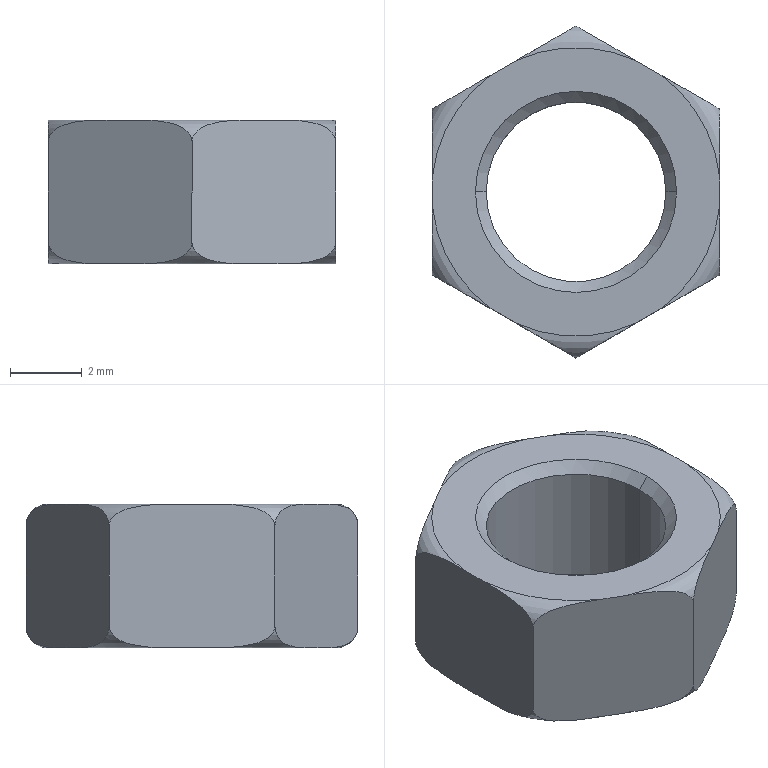Part | NX | features BREP 1 | 1 solid | 26 faces | box 8 x 9.238 x 4 mm | volume 141.214 mm3 | torus 12 | plane 8 | cone 4 | cylinder 2 | commonest cylinder face diameters 5 x2
STEP:
#1=CARTESIAN_POINT('',(2.5,0.,-1.7));
#2=VERTEX_POINT('',#1);
#3=CARTESIAN_POINT('',(-2.5,0.,-1.7));
#4=VERTEX_POINT('',#3);
#5=CARTESIAN_POINT('',(0.,0.,-1.7));
#6=DIRECTION('',(0.,0.,-1.));
#7=DIRECTION('',(-1.,0.,0.));
#8=AXIS2_PLACEMENT_3D('',#5,#6,#7);
#9=CIRCLE('',#8,2.5);
#10=EDGE_CURVE('',#2,#4,#9,.T.);
#11=ORIENTED_EDGE('',*,*,#10,.F.);
#12=CARTESIAN_POINT('',(2.8,0.,-2.));
#13=VERTEX_POINT('',#12);
#14=CARTESIAN_POINT('',(2.8,0.,-2.));
#15=DIRECTION('',(0.7071,0.,-0.7071));
#16=VECTOR('',#15,1000.);
#17=LINE('',#14,#16);
#18=EDGE_CURVE('',#2,#13,#17,.T.);
#19=ORIENTED_EDGE('',*,*,#18,.T.);
#20=CARTESIAN_POINT('',(-2.8,0.,-2.));
#21=VERTEX_POINT('',#20);
#22=CARTESIAN_POINT('',(0.,0.,-2.));
#23=DIRECTION('',(0.,0.,-1.));
#24=DIRECTION('',(-1.,0.,0.));
#25=AXIS2_PLACEMENT_3D('',#22,#23,#24);
#26=CIRCLE('',#25,2.8);
#27=EDGE_CURVE('',#13,#21,#26,.T.);
#28=ORIENTED_EDGE('',*,*,#27,.T.);
#29=CARTESIAN_POINT('',(-2.8,0.,-2.));
#30=DIRECTION('',(-0.7071,0.,-0.7071));
#31=VECTOR('',#30,1000.);
#32=LINE('',#29,#31);
#33=EDGE_CURVE('',#4,#21,#32,.T.);
#34=ORIENTED_EDGE('',*,*,#33,.F.);
#35=EDGE_LOOP('',(#11,#19,#28,#34));
#36=FACE_BOUND('',#35,.T.);
#37=CARTESIAN_POINT('',(0.,0.,-2.));
#38=DIRECTION('',(0.,0.,-1.));
#39=DIRECTION('',(-1.,0.,0.));
#40=AXIS2_PLACEMENT_3D('',#37,#38,#39);
#41=CONICAL_SURFACE('',#40,2.8,0.7854);
#42=ADVANCED_FACE('',(#36),#41,.F.);
#43=CARTESIAN_POINT('',(2.5,0.,1.7));
#44=VERTEX_POINT('',#43);
#45=CARTESIAN_POINT('',(-2.5,0.,1.7));
#46=VERTEX_POINT('',#45);
#47=CARTESIAN_POINT('',(0.,0.,1.7));
#48=DIRECTION('',(0.,0.,-1.));
#49=DIRECTION('',(-1.,0.,0.));
#50=AXIS2_PLACEMENT_3D('',#47,#48,#49);
#51=CIRCLE('',#50,2.5);
#52=EDGE_CURVE('',#44,#46,#51,.T.);
#53=ORIENTED_EDGE('',*,*,#52,.T.);
#54=CARTESIAN_POINT('',(-2.8,0.,2.));
#55=VERTEX_POINT('',#54);
#56=CARTESIAN_POINT('',(-2.5,0.,1.7));
#57=DIRECTION('',(-0.7071,0.,0.7071));
#58=VECTOR('',#57,1000.);
#59=LINE('',#56,#58);
#60=EDGE_CURVE('',#55,#46,#59,.F.);
#61=ORIENTED_EDGE('',*,*,#60,.F.);
#62=CARTESIAN_POINT('',(2.8,0.,2.));
#63=VERTEX_POINT('',#62);
#64=CARTESIAN_POINT('',(0.,0.,2.));
#65=DIRECTION('',(0.,0.,-1.));
#66=DIRECTION('',(-1.,0.,0.));
#67=AXIS2_PLACEMENT_3D('',#64,#65,#66);
#68=CIRCLE('',#67,2.8);
#69=EDGE_CURVE('',#63,#55,#68,.T.);
#70=ORIENTED_EDGE('',*,*,#69,.F.);
#71=CARTESIAN_POINT('',(2.5,0.,1.7));
#72=DIRECTION('',(0.7071,0.,0.7071));
#73=VECTOR('',#72,1000.);
#74=LINE('',#71,#73);
#75=EDGE_CURVE('',#63,#44,#74,.F.);
#76=ORIENTED_EDGE('',*,*,#75,.T.);
#77=EDGE_LOOP('',(#53,#61,#70,#76));
#78=FACE_BOUND('',#77,.T.);
#79=CARTESIAN_POINT('',(0.,0.,1.7));
#80=DIRECTION('',(0.,0.,1.));
#81=DIRECTION('',(1.,0.,0.));
#82=AXIS2_PLACEMENT_3D('',#79,#80,#81);
#83=CONICAL_SURFACE('',#82,2.5,0.7854);
#84=ADVANCED_FACE('',(#78),#83,.F.);
#85=ORIENTED_EDGE('',*,*,#52,.F.);
#86=CARTESIAN_POINT('',(2.5,0.,2.));
#87=DIRECTION('',(0.,0.,-1.));
#88=VECTOR('',#87,1000.);
#89=LINE('',#86,#88);
#90=EDGE_CURVE('',#44,#2,#89,.T.);
#91=ORIENTED_EDGE('',*,*,#90,.T.);
#92=ORIENTED_EDGE('',*,*,#10,.T.);
#93=CARTESIAN_POINT('',(-2.5,0.,2.));
#94=DIRECTION('',(0.,0.,-1.));
#95=VECTOR('',#94,1000.);
#96=LINE('',#93,#95);
#97=EDGE_CURVE('',#46,#4,#96,.T.);
#98=ORIENTED_EDGE('',*,*,#97,.F.);
#99=EDGE_LOOP('',(#85,#91,#92,#98));
#100=FACE_BOUND('',#99,.T.);
#101=CARTESIAN_POINT('',(0.,0.,2.));
#102=DIRECTION('',(0.,0.,-1.));
#103=DIRECTION('',(-1.,0.,0.));
#104=AXIS2_PLACEMENT_3D('',#101,#102,#103);
#105=CYLINDRICAL_SURFACE('',#104,2.5);
#106=ADVANCED_FACE('',(#100),#105,.F.);
#107=CARTESIAN_POINT('',(-2.336,-3.27,-2.));
#108=VERTEX_POINT('',#107);
#109=CARTESIAN_POINT('',(-4.,-0.3883,-2.));
#110=VERTEX_POINT('',#109);
#111=CARTESIAN_POINT('',(0.,0.,-2.));
#112=DIRECTION('',(0.,0.,-1.));
#113=DIRECTION('',(-1.,0.,0.));
#114=AXIS2_PLACEMENT_3D('',#111,#112,#113);
#115=CIRCLE('',#114,4.019);
#116=EDGE_CURVE('',#108,#110,#115,.T.);
#117=ORIENTED_EDGE('',*,*,#116,.T.);
#118=CARTESIAN_POINT('',(-4.,0.3883,-2.));
#119=VERTEX_POINT('',#118);
#120=CARTESIAN_POINT('',(-4.,2.309,-2.));
#121=DIRECTION('',(0.,-1.,0.));
#122=VECTOR('',#121,1000.);
#123=LINE('',#120,#122);
#124=EDGE_CURVE('',#119,#110,#123,.T.);
#125=ORIENTED_EDGE('',*,*,#124,.F.);
#126=CARTESIAN_POINT('',(-2.336,3.27,-2.));
#127=VERTEX_POINT('',#126);
#128=CARTESIAN_POINT('',(0.,0.,-2.));
#129=DIRECTION('',(0.,0.,-1.));
#130=DIRECTION('',(-1.,0.,0.));
#131=AXIS2_PLACEMENT_3D('',#128,#129,#130);
#132=CIRCLE('',#131,4.019);
#133=EDGE_CURVE('',#119,#127,#132,.T.);
#134=ORIENTED_EDGE('',*,*,#133,.T.);
#135=CARTESIAN_POINT('',(-1.664,3.658,-2.));
#136=VERTEX_POINT('',#135);
#137=CARTESIAN_POINT('',(0.,4.619,-2.));
#138=DIRECTION('',(-0.866,-0.5,0.));
#139=VECTOR('',#138,1000.);
#140=LINE('',#137,#139);
#141=EDGE_CURVE('',#136,#127,#140,.T.);
#142=ORIENTED_EDGE('',*,*,#141,.F.);
#143=CARTESIAN_POINT('',(1.664,3.658,-2.));
#144=VERTEX_POINT('',#143);
#145=CARTESIAN_POINT('',(0.,0.,-2.));
#146=DIRECTION('',(0.,0.,-1.));
#147=DIRECTION('',(-1.,0.,0.));
#148=AXIS2_PLACEMENT_3D('',#145,#146,#147);
#149=CIRCLE('',#148,4.019);
#150=EDGE_CURVE('',#136,#144,#149,.T.);
#151=ORIENTED_EDGE('',*,*,#150,.T.);
#152=CARTESIAN_POINT('',(2.336,3.27,-2.));
#153=VERTEX_POINT('',#152);
#154=CARTESIAN_POINT('',(4.,2.309,-2.));
#155=DIRECTION('',(-0.866,0.5,0.));
#156=VECTOR('',#155,1000.);
#157=LINE('',#154,#156);
#158=EDGE_CURVE('',#153,#144,#157,.T.);
#159=ORIENTED_EDGE('',*,*,#158,.F.);
#160=CARTESIAN_POINT('',(4.,0.3883,-2.));
#161=VERTEX_POINT('',#160);
#162=CARTESIAN_POINT('',(0.,0.,-2.));
#163=DIRECTION('',(0.,0.,-1.));
#164=DIRECTION('',(-1.,0.,0.));
#165=AXIS2_PLACEMENT_3D('',#162,#163,#164);
#166=CIRCLE('',#165,4.019);
#167=EDGE_CURVE('',#153,#161,#166,.T.);
#168=ORIENTED_EDGE('',*,*,#167,.T.);
#169=CARTESIAN_POINT('',(4.,-0.3883,-2.));
#170=VERTEX_POINT('',#169);
#171=CARTESIAN_POINT('',(4.,-2.309,-2.));
#172=DIRECTION('',(0.,1.,0.));
#173=VECTOR('',#172,1000.);
#174=LINE('',#171,#173);
#175=EDGE_CURVE('',#170,#161,#174,.T.);
#176=ORIENTED_EDGE('',*,*,#175,.F.);
#177=CARTESIAN_POINT('',(2.336,-3.27,-2.));
#178=VERTEX_POINT('',#177);
#179=CARTESIAN_POINT('',(0.,0.,-2.));
#180=DIRECTION('',(0.,0.,-1.));
#181=DIRECTION('',(-1.,0.,0.));
#182=AXIS2_PLACEMENT_3D('',#179,#180,#181);
#183=CIRCLE('',#182,4.019);
#184=EDGE_CURVE('',#170,#178,#183,.T.);
#185=ORIENTED_EDGE('',*,*,#184,.T.);
#186=CARTESIAN_POINT('',(1.664,-3.658,-2.));
#187=VERTEX_POINT('',#186);
#188=CARTESIAN_POINT('',(0.,-4.619,-2.));
#189=DIRECTION('',(0.866,0.5,0.));
#190=VECTOR('',#189,1000.);
#191=LINE('',#188,#190);
#192=EDGE_CURVE('',#187,#178,#191,.T.);
#193=ORIENTED_EDGE('',*,*,#192,.F.);
#194=CARTESIAN_POINT('',(-1.664,-3.658,-2.));
#195=VERTEX_POINT('',#194);
#196=CARTESIAN_POINT('',(0.,0.,-2.));
#197=DIRECTION('',(0.,0.,-1.));
#198=DIRECTION('',(-1.,0.,0.));
#199=AXIS2_PLACEMENT_3D('',#196,#197,#198);
#200=CIRCLE('',#199,4.019);
#201=EDGE_CURVE('',#187,#195,#200,.T.);
#202=ORIENTED_EDGE('',*,*,#201,.T.);
#203=CARTESIAN_POINT('',(-4.,-2.309,-2.));
#204=DIRECTION('',(0.866,-0.5,0.));
#205=VECTOR('',#204,1000.);
#206=LINE('',#203,#205);
#207=EDGE_CURVE('',#108,#195,#206,.T.);
#208=ORIENTED_EDGE('',*,*,#207,.F.);
#209=EDGE_LOOP('',(#117,#125,#134,#142,#151,#159,#168,#176,#185,#193,#202,#208));
#210=FACE_BOUND('',#209,.T.);
#211=CARTESIAN_POINT('',(0.,0.,-2.));
#212=DIRECTION('',(0.,0.,-1.));
#213=DIRECTION('',(-1.,0.,0.));
#214=AXIS2_PLACEMENT_3D('',#211,#212,#213);
#215=CIRCLE('',#214,2.8);
#216=EDGE_CURVE('',#21,#13,#215,.T.);
#217=ORIENTED_EDGE('',*,*,#216,.F.);
#218=ORIENTED_EDGE('',*,*,#27,.F.);
#219=EDGE_LOOP('',(#217,#218));
#220=FACE_BOUND('',#219,.T.);
#221=CARTESIAN_POINT('',(-4.,6.928,-2.));
#222=DIRECTION('',(0.,0.,1.));
#223=DIRECTION('',(1.,0.,0.));
#224=AXIS2_PLACEMENT_3D('',#221,#222,#223);
#225=PLANE('',#224);
#226=ADVANCED_FACE('',(#210,#220),#225,.F.);
#227=CARTESIAN_POINT('',(-4.,0.3883,2.));
#228=VERTEX_POINT('',#227);
#229=CARTESIAN_POINT('',(-4.,-0.3883,2.));
#230=VERTEX_POINT('',#229);
#231=CARTESIAN_POINT('',(-4.,2.309,2.));
#232=DIRECTION('',(0.,-1.,0.));
#233=VECTOR('',#232,1000.);
#234=LINE('',#231,#233);
#235=EDGE_CURVE('',#228,#230,#234,.T.);
#236=ORIENTED_EDGE('',*,*,#235,.T.);
#237=CARTESIAN_POINT('',(-2.336,-3.27,2.));
#238=VERTEX_POINT('',#237);
#239=CARTESIAN_POINT('',(0.,0.,2.));
#240=DIRECTION('',(0.,0.,-1.));
#241=DIRECTION('',(-1.,0.,0.));
#242=AXIS2_PLACEMENT_3D('',#239,#240,#241);
#243=CIRCLE('',#242,4.019);
#244=EDGE_CURVE('',#238,#230,#243,.T.);
#245=ORIENTED_EDGE('',*,*,#244,.F.);
#246=CARTESIAN_POINT('',(-1.664,-3.658,2.));
#247=VERTEX_POINT('',#246);
#248=CARTESIAN_POINT('',(-4.,-2.309,2.));
#249=DIRECTION('',(0.866,-0.5,0.));
#250=VECTOR('',#249,1000.);
#251=LINE('',#248,#250);
#252=EDGE_CURVE('',#238,#247,#251,.T.);
#253=ORIENTED_EDGE('',*,*,#252,.T.);
#254=CARTESIAN_POINT('',(1.664,-3.658,2.));
#255=VERTEX_POINT('',#254);
#256=CARTESIAN_POINT('',(0.,0.,2.));
#257=DIRECTION('',(0.,0.,-1.));
#258=DIRECTION('',(-1.,0.,0.));
#259=AXIS2_PLACEMENT_3D('',#256,#257,#258);
#260=CIRCLE('',#259,4.019);
#261=EDGE_CURVE('',#255,#247,#260,.T.);
#262=ORIENTED_EDGE('',*,*,#261,.F.);
#263=CARTESIAN_POINT('',(2.336,-3.27,2.));
#264=VERTEX_POINT('',#263);
#265=CARTESIAN_POINT('',(0.,-4.619,2.));
#266=DIRECTION('',(0.866,0.5,0.));
#267=VECTOR('',#266,1000.);
#268=LINE('',#265,#267);
#269=EDGE_CURVE('',#255,#264,#268,.T.);
#270=ORIENTED_EDGE('',*,*,#269,.T.);
#271=CARTESIAN_POINT('',(4.,-0.3883,2.));
#272=VERTEX_POINT('',#271);
#273=CARTESIAN_POINT('',(0.,0.,2.));
#274=DIRECTION('',(0.,0.,-1.));
#275=DIRECTION('',(-1.,0.,0.));
#276=AXIS2_PLACEMENT_3D('',#273,#274,#275);
#277=CIRCLE('',#276,4.019);
#278=EDGE_CURVE('',#272,#264,#277,.T.);
#279=ORIENTED_EDGE('',*,*,#278,.F.);
#280=CARTESIAN_POINT('',(4.,0.3883,2.));
#281=VERTEX_POINT('',#280);
#282=CARTESIAN_POINT('',(4.,-2.309,2.));
#283=DIRECTION('',(0.,1.,0.));
#284=VECTOR('',#283,1000.);
#285=LINE('',#282,#284);
#286=EDGE_CURVE('',#272,#281,#285,.T.);
#287=ORIENTED_EDGE('',*,*,#286,.T.);
#288=CARTESIAN_POINT('',(2.336,3.27,2.));
#289=VERTEX_POINT('',#288);
#290=CARTESIAN_POINT('',(0.,0.,2.));
#291=DIRECTION('',(0.,0.,-1.));
#292=DIRECTION('',(-1.,0.,0.));
#293=AXIS2_PLACEMENT_3D('',#290,#291,#292);
#294=CIRCLE('',#293,4.019);
#295=EDGE_CURVE('',#289,#281,#294,.T.);
#296=ORIENTED_EDGE('',*,*,#295,.F.);
#297=CARTESIAN_POINT('',(1.664,3.658,2.));
#298=VERTEX_POINT('',#297);
#299=CARTESIAN_POINT('',(4.,2.309,2.));
#300=DIRECTION('',(-0.866,0.5,0.));
#301=VECTOR('',#300,1000.);
#302=LINE('',#299,#301);
#303=EDGE_CURVE('',#289,#298,#302,.T.);
#304=ORIENTED_EDGE('',*,*,#303,.T.);
#305=CARTESIAN_POINT('',(-1.664,3.658,2.));
#306=VERTEX_POINT('',#305);
#307=CARTESIAN_POINT('',(0.,0.,2.));
#308=DIRECTION('',(0.,0.,-1.));
#309=DIRECTION('',(-1.,0.,0.));
#310=AXIS2_PLACEMENT_3D('',#307,#308,#309);
#311=CIRCLE('',#310,4.019);
#312=EDGE_CURVE('',#306,#298,#311,.T.);
#313=ORIENTED_EDGE('',*,*,#312,.F.);
#314=CARTESIAN_POINT('',(-2.336,3.27,2.));
#315=VERTEX_POINT('',#314);
#316=CARTESIAN_POINT('',(0.,4.619,2.));
#317=DIRECTION('',(-0.866,-0.5,0.));
#318=VECTOR('',#317,1000.);
#319=LINE('',#316,#318);
#320=EDGE_CURVE('',#306,#315,#319,.T.);
#321=ORIENTED_EDGE('',*,*,#320,.T.);
#322=CARTESIAN_POINT('',(0.,0.,2.));
#323=DIRECTION('',(0.,0.,-1.));
#324=DIRECTION('',(-1.,0.,0.));
#325=AXIS2_PLACEMENT_3D('',#322,#323,#324);
#326=CIRCLE('',#325,4.019);
#327=EDGE_CURVE('',#228,#315,#326,.T.);
#328=ORIENTED_EDGE('',*,*,#327,.F.);
#329=EDGE_LOOP('',(#236,#245,#253,#262,#270,#279,#287,#296,#304,#313,#321,#328));
#330=FACE_BOUND('',#329,.T.);
#331=ORIENTED_EDGE('',*,*,#69,.T.);
#332=CARTESIAN_POINT('',(0.,0.,2.));
#333=DIRECTION('',(0.,0.,-1.));
#334=DIRECTION('',(-1.,0.,0.));
#335=AXIS2_PLACEMENT_3D('',#332,#333,#334);
#336=CIRCLE('',#335,2.8);
#337=EDGE_CURVE('',#55,#63,#336,.T.);
#338=ORIENTED_EDGE('',*,*,#337,.T.);
#339=EDGE_LOOP('',(#331,#338));
#340=FACE_BOUND('',#339,.T.);
#341=CARTESIAN_POINT('',(-4.,6.928,2.));
#342=DIRECTION('',(0.,0.,1.));
#343=DIRECTION('',(1.,0.,0.));
#344=AXIS2_PLACEMENT_3D('',#341,#342,#343);
#345=PLANE('',#344);
#346=ADVANCED_FACE('',(#330,#340),#345,.T.);
#347=CARTESIAN_POINT('',(4.,2.309,1.4));
#348=VERTEX_POINT('',#347);
#349=CARTESIAN_POINT('',(4.,2.309,-1.4));
#350=VERTEX_POINT('',#349);
#351=CARTESIAN_POINT('',(4.,2.309,2.));
#352=DIRECTION('',(0.,0.,-1.));
#353=VECTOR('',#352,1000.);
#354=LINE('',#351,#353);
#355=EDGE_CURVE('',#348,#350,#354,.T.);
#356=ORIENTED_EDGE('',*,*,#355,.T.);
#357=CARTESIAN_POINT('',(4.,2.309,-1.4));
#358=CARTESIAN_POINT('',(4.,2.309,-1.575));
#359=CARTESIAN_POINT('',(3.769,2.443,-1.795));
#360=CARTESIAN_POINT('',(3.536,2.578,-1.889));
#361=CARTESIAN_POINT('',(3.249,2.743,-1.958));
#362=CARTESIAN_POINT('',(3.077,2.842,-1.977));
#363=CARTESIAN_POINT('',(2.78,3.014,-1.996));
#364=CARTESIAN_POINT('',(2.625,3.103,-1.998));
#365=CARTESIAN_POINT('',(2.437,3.212,-2.));
#366=CARTESIAN_POINT('',(2.336,3.27,-2.));
#367=B_SPLINE_CURVE_WITH_KNOTS('',3,(#357,#358,#359,#360,#361,#362,#363,#364,#365,#366),.UNSPECIFIED.,.F.,.F.,(4,1,1,1,1,1,1,4),(0.,0.25,0.375,0.5,0.625,0.75,0.875,1.),.UNSPECIFIED.);
#368=EDGE_CURVE('',#350,#153,#367,.T.);
#369=ORIENTED_EDGE('',*,*,#368,.T.);
#370=ORIENTED_EDGE('',*,*,#158,.T.);
#371=CARTESIAN_POINT('',(0.,4.619,-1.4));
#372=VERTEX_POINT('',#371);
#373=CARTESIAN_POINT('',(1.664,3.658,-2.));
#374=CARTESIAN_POINT('',(1.463,3.774,-2.));
#375=CARTESIAN_POINT('',(1.304,3.866,-2.002));
#376=CARTESIAN_POINT('',(0.9254,4.085,-1.978));
#377=CARTESIAN_POINT('',(0.7461,4.188,-1.957));
#378=CARTESIAN_POINT('',(0.4638,4.351,-1.889));
#379=CARTESIAN_POINT('',(0.2273,4.488,-1.792));
#380=CARTESIAN_POINT('',(0.,4.619,-1.577));
#381=CARTESIAN_POINT('',(0.,4.619,-1.4));
#382=B_SPLINE_CURVE_WITH_KNOTS('',3,(#373,#374,#375,#376,#377,#378,#379,#380,#381),.UNSPECIFIED.,.F.,.F.,(4,1,1,1,1,1,4),(0.,0.25,0.375,0.5,0.625,0.75,1.),.UNSPECIFIED.);
#383=EDGE_CURVE('',#144,#372,#382,.T.);
#384=ORIENTED_EDGE('',*,*,#383,.T.);
#385=CARTESIAN_POINT('',(0.,4.619,1.4));
#386=VERTEX_POINT('',#385);
#387=CARTESIAN_POINT('',(0.,4.619,2.));
#388=DIRECTION('',(0.,0.,-1.));
#389=VECTOR('',#388,1000.);
#390=LINE('',#387,#389);
#391=EDGE_CURVE('',#386,#372,#390,.T.);
#392=ORIENTED_EDGE('',*,*,#391,.F.);
#393=CARTESIAN_POINT('',(0.,4.619,1.4));
#394=CARTESIAN_POINT('',(0.,4.619,1.575));
#395=CARTESIAN_POINT('',(0.2312,4.485,1.795));
#396=CARTESIAN_POINT('',(0.4644,4.351,1.889));
#397=CARTESIAN_POINT('',(0.7506,4.185,1.958));
#398=CARTESIAN_POINT('',(0.9231,4.086,1.977));
#399=CARTESIAN_POINT('',(1.22,3.915,1.996));
#400=CARTESIAN_POINT('',(1.375,3.825,1.998));
#401=CARTESIAN_POINT('',(1.563,3.716,2.));
#402=CARTESIAN_POINT('',(1.664,3.658,2.));
#403=B_SPLINE_CURVE_WITH_KNOTS('',3,(#393,#394,#395,#396,#397,#398,#399,#400,#401,#402),.UNSPECIFIED.,.F.,.F.,(4,1,1,1,1,1,1,4),(0.,0.25,0.375,0.5,0.625,0.75,0.875,1.),.UNSPECIFIED.);
#404=EDGE_CURVE('',#386,#298,#403,.T.);
#405=ORIENTED_EDGE('',*,*,#404,.T.);
#406=ORIENTED_EDGE('',*,*,#303,.F.);
#407=CARTESIAN_POINT('',(2.336,3.27,2.));
#408=CARTESIAN_POINT('',(2.537,3.154,2.));
#409=CARTESIAN_POINT('',(2.696,3.062,2.002));
#410=CARTESIAN_POINT('',(3.075,2.844,1.978));
#411=CARTESIAN_POINT('',(3.254,2.74,1.957));
#412=CARTESIAN_POINT('',(3.536,2.577,1.889));
#413=CARTESIAN_POINT('',(3.773,2.441,1.792));
#414=CARTESIAN_POINT('',(4.,2.309,1.577));
#415=CARTESIAN_POINT('',(4.,2.309,1.4));
#416=B_SPLINE_CURVE_WITH_KNOTS('',3,(#407,#408,#409,#410,#411,#412,#413,#414,#415),.UNSPECIFIED.,.F.,.F.,(4,1,1,1,1,1,4),(0.,0.25,0.375,0.5,0.625,0.75,1.),.UNSPECIFIED.);
#417=EDGE_CURVE('',#289,#348,#416,.T.);
#418=ORIENTED_EDGE('',*,*,#417,.T.);
#419=EDGE_LOOP('',(#356,#369,#370,#384,#392,#405,#406,#418));
#420=FACE_BOUND('',#419,.T.);
#421=CARTESIAN_POINT('',(4.,2.309,2.));
#422=DIRECTION('',(-0.5,-0.866,0.));
#423=DIRECTION('',(-0.866,0.5,0.));
#424=AXIS2_PLACEMENT_3D('',#421,#422,#423);
#425=PLANE('',#424);
#426=ADVANCED_FACE('',(#420),#425,.F.);
#427=ORIENTED_EDGE('',*,*,#391,.T.);
#428=CARTESIAN_POINT('',(0.,4.619,-1.4));
#429=CARTESIAN_POINT('',(0.,4.619,-1.575));
#430=CARTESIAN_POINT('',(-0.2312,4.485,-1.795));
#431=CARTESIAN_POINT('',(-0.4644,4.351,-1.889));
#432=CARTESIAN_POINT('',(-0.7506,4.185,-1.958));
#433=CARTESIAN_POINT('',(-0.9231,4.086,-1.977));
#434=CARTESIAN_POINT('',(-1.22,3.915,-1.996));
#435=CARTESIAN_POINT('',(-1.375,3.825,-1.998));
#436=CARTESIAN_POINT('',(-1.563,3.716,-2.));
#437=CARTESIAN_POINT('',(-1.664,3.658,-2.));
#438=B_SPLINE_CURVE_WITH_KNOTS('',3,(#428,#429,#430,#431,#432,#433,#434,#435,#436,#437),.UNSPECIFIED.,.F.,.F.,(4,1,1,1,1,1,1,4),(0.,0.25,0.375,0.5,0.625,0.75,0.875,1.),.UNSPECIFIED.);
#439=EDGE_CURVE('',#372,#136,#438,.T.);
#440=ORIENTED_EDGE('',*,*,#439,.T.);
#441=ORIENTED_EDGE('',*,*,#141,.T.);
#442=CARTESIAN_POINT('',(-4.,2.309,-1.4));
#443=VERTEX_POINT('',#442);
#444=CARTESIAN_POINT('',(-2.336,3.27,-2.));
#445=CARTESIAN_POINT('',(-2.537,3.154,-2.));
#446=CARTESIAN_POINT('',(-2.696,3.062,-2.002));
#447=CARTESIAN_POINT('',(-3.075,2.844,-1.978));
#448=CARTESIAN_POINT('',(-3.254,2.74,-1.957));
#449=CARTESIAN_POINT('',(-3.536,2.577,-1.889));
#450=CARTESIAN_POINT('',(-3.773,2.441,-1.792));
#451=CARTESIAN_POINT('',(-4.,2.309,-1.577));
#452=CARTESIAN_POINT('',(-4.,2.309,-1.4));
#453=B_SPLINE_CURVE_WITH_KNOTS('',3,(#444,#445,#446,#447,#448,#449,#450,#451,#452),.UNSPECIFIED.,.F.,.F.,(4,1,1,1,1,1,4),(0.,0.25,0.375,0.5,0.625,0.75,1.),.UNSPECIFIED.);
#454=EDGE_CURVE('',#127,#443,#453,.T.);
#455=ORIENTED_EDGE('',*,*,#454,.T.);
#456=CARTESIAN_POINT('',(-4.,2.309,1.4));
#457=VERTEX_POINT('',#456);
#458=CARTESIAN_POINT('',(-4.,2.309,2.));
#459=DIRECTION('',(0.,0.,-1.));
#460=VECTOR('',#459,1000.);
#461=LINE('',#458,#460);
#462=EDGE_CURVE('',#457,#443,#461,.T.);
#463=ORIENTED_EDGE('',*,*,#462,.F.);
#464=CARTESIAN_POINT('',(-4.,2.309,1.4));
#465=CARTESIAN_POINT('',(-4.,2.309,1.575));
#466=CARTESIAN_POINT('',(-3.769,2.443,1.795));
#467=CARTESIAN_POINT('',(-3.536,2.578,1.889));
#468=CARTESIAN_POINT('',(-3.249,2.743,1.958));
#469=CARTESIAN_POINT('',(-3.077,2.842,1.977));
#470=CARTESIAN_POINT('',(-2.78,3.014,1.996));
#471=CARTESIAN_POINT('',(-2.625,3.103,1.998));
#472=CARTESIAN_POINT('',(-2.437,3.212,2.));
#473=CARTESIAN_POINT('',(-2.336,3.27,2.));
#474=B_SPLINE_CURVE_WITH_KNOTS('',3,(#464,#465,#466,#467,#468,#469,#470,#471,#472,#473),.UNSPECIFIED.,.F.,.F.,(4,1,1,1,1,1,1,4),(0.,0.25,0.375,0.5,0.625,0.75,0.875,1.),.UNSPECIFIED.);
#475=EDGE_CURVE('',#457,#315,#474,.T.);
#476=ORIENTED_EDGE('',*,*,#475,.T.);
#477=ORIENTED_EDGE('',*,*,#320,.F.);
#478=CARTESIAN_POINT('',(-1.664,3.658,2.));
#479=CARTESIAN_POINT('',(-1.463,3.774,2.));
#480=CARTESIAN_POINT('',(-1.304,3.866,2.002));
#481=CARTESIAN_POINT('',(-0.9254,4.085,1.978));
#482=CARTESIAN_POINT('',(-0.7461,4.188,1.957));
#483=CARTESIAN_POINT('',(-0.4638,4.351,1.889));
#484=CARTESIAN_POINT('',(-0.2273,4.488,1.792));
#485=CARTESIAN_POINT('',(0.,4.619,1.577));
#486=CARTESIAN_POINT('',(0.,4.619,1.4));
#487=B_SPLINE_CURVE_WITH_KNOTS('',3,(#478,#479,#480,#481,#482,#483,#484,#485,#486),.UNSPECIFIED.,.F.,.F.,(4,1,1,1,1,1,4),(0.,0.25,0.375,0.5,0.625,0.75,1.),.UNSPECIFIED.);
#488=EDGE_CURVE('',#306,#386,#487,.T.);
#489=ORIENTED_EDGE('',*,*,#488,.T.);
#490=EDGE_LOOP('',(#427,#440,#441,#455,#463,#476,#477,#489));
#491=FACE_BOUND('',#490,.T.);
#492=CARTESIAN_POINT('',(0.,4.619,2.));
#493=DIRECTION('',(0.5,-0.866,0.));
#494=DIRECTION('',(0.,0.,-1.));
#495=AXIS2_PLACEMENT_3D('',#492,#493,#494);
#496=PLANE('',#495);
#497=ADVANCED_FACE('',(#491),#496,.F.);
#498=ORIENTED_EDGE('',*,*,#124,.T.);
#499=CARTESIAN_POINT('',(-4.,-2.309,-1.4));
#500=VERTEX_POINT('',#499);
#501=CARTESIAN_POINT('',(-4.,-0.3883,-2.));
#502=CARTESIAN_POINT('',(-4.,-0.6198,-2.));
#503=CARTESIAN_POINT('',(-4.,-0.8035,-2.002));
#504=CARTESIAN_POINT('',(-4.,-1.24,-1.978));
#505=CARTESIAN_POINT('',(-4.,-1.447,-1.957));
#506=CARTESIAN_POINT('',(-4.,-1.774,-1.889));
#507=CARTESIAN_POINT('',(-4.,-2.047,-1.793));
#508=CARTESIAN_POINT('',(-4.,-2.309,-1.573));
#509=CARTESIAN_POINT('',(-4.,-2.309,-1.4));
#510=B_SPLINE_CURVE_WITH_KNOTS('',3,(#501,#502,#503,#504,#505,#506,#507,#508,#509),.UNSPECIFIED.,.F.,.F.,(4,1,1,1,1,1,4),(0.,0.25,0.375,0.5,0.625,0.75,1.),.UNSPECIFIED.);
#511=EDGE_CURVE('',#110,#500,#510,.T.);
#512=ORIENTED_EDGE('',*,*,#511,.T.);
#513=CARTESIAN_POINT('',(-4.,-2.309,1.4));
#514=VERTEX_POINT('',#513);
#515=CARTESIAN_POINT('',(-4.,-2.309,2.));
#516=DIRECTION('',(0.,0.,-1.));
#517=VECTOR('',#516,1000.);
#518=LINE('',#515,#517);
#519=EDGE_CURVE('',#514,#500,#518,.T.);
#520=ORIENTED_EDGE('',*,*,#519,.F.);
#521=CARTESIAN_POINT('',(-4.,-2.309,1.4));
#522=CARTESIAN_POINT('',(-4.,-2.309,1.573));
#523=CARTESIAN_POINT('',(-4.,-2.041,1.796));
#524=CARTESIAN_POINT('',(-4.,-1.771,1.89));
#525=CARTESIAN_POINT('',(-4.,-1.438,1.958));
#526=CARTESIAN_POINT('',(-4.,-1.241,1.978));
#527=CARTESIAN_POINT('',(-4.,-0.8989,1.997));
#528=CARTESIAN_POINT('',(-4.,-0.7208,1.998));
#529=CARTESIAN_POINT('',(-4.,-0.504,2.));
#530=CARTESIAN_POINT('',(-4.,-0.3883,2.));
#531=B_SPLINE_CURVE_WITH_KNOTS('',3,(#521,#522,#523,#524,#525,#526,#527,#528,#529,#530),.UNSPECIFIED.,.F.,.F.,(4,1,1,1,1,1,1,4),(0.,0.25,0.375,0.5,0.625,0.75,0.875,1.),.UNSPECIFIED.);
#532=EDGE_CURVE('',#514,#230,#531,.T.);
#533=ORIENTED_EDGE('',*,*,#532,.T.);
#534=ORIENTED_EDGE('',*,*,#235,.F.);
#535=CARTESIAN_POINT('',(-4.,0.3883,2.));
#536=CARTESIAN_POINT('',(-4.,0.6198,2.));
#537=CARTESIAN_POINT('',(-4.,0.8035,2.002));
#538=CARTESIAN_POINT('',(-4.,1.24,1.978));
#539=CARTESIAN_POINT('',(-4.,1.447,1.957));
#540=CARTESIAN_POINT('',(-4.,1.774,1.889));
#541=CARTESIAN_POINT('',(-4.,2.047,1.793));
#542=CARTESIAN_POINT('',(-4.,2.309,1.573));
#543=CARTESIAN_POINT('',(-4.,2.309,1.4));
#544=B_SPLINE_CURVE_WITH_KNOTS('',3,(#535,#536,#537,#538,#539,#540,#541,#542,#543),.UNSPECIFIED.,.F.,.F.,(4,1,1,1,1,1,4),(0.,0.25,0.375,0.5,0.625,0.75,1.),.UNSPECIFIED.);
#545=EDGE_CURVE('',#228,#457,#544,.T.);
#546=ORIENTED_EDGE('',*,*,#545,.T.);
#547=ORIENTED_EDGE('',*,*,#462,.T.);
#548=CARTESIAN_POINT('',(-4.,2.309,-1.4));
#549=CARTESIAN_POINT('',(-4.,2.309,-1.573));
#550=CARTESIAN_POINT('',(-4.,2.041,-1.796));
#551=CARTESIAN_POINT('',(-4.,1.771,-1.89));
#552=CARTESIAN_POINT('',(-4.,1.438,-1.958));
#553=CARTESIAN_POINT('',(-4.,1.241,-1.978));
#554=CARTESIAN_POINT('',(-4.,0.8989,-1.997));
#555=CARTESIAN_POINT('',(-4.,0.7208,-1.998));
#556=CARTESIAN_POINT('',(-4.,0.504,-2.));
#557=CARTESIAN_POINT('',(-4.,0.3883,-2.));
#558=B_SPLINE_CURVE_WITH_KNOTS('',3,(#548,#549,#550,#551,#552,#553,#554,#555,#556,#557),.UNSPECIFIED.,.F.,.F.,(4,1,1,1,1,1,1,4),(0.,0.25,0.375,0.5,0.625,0.75,0.875,1.),.UNSPECIFIED.);
#559=EDGE_CURVE('',#443,#119,#558,.T.);
#560=ORIENTED_EDGE('',*,*,#559,.T.);
#561=EDGE_LOOP('',(#498,#512,#520,#533,#534,#546,#547,#560));
#562=FACE_BOUND('',#561,.T.);
#563=CARTESIAN_POINT('',(-4.,2.309,2.));
#564=DIRECTION('',(1.,0.,0.));
#565=DIRECTION('',(0.,1.,0.));
#566=AXIS2_PLACEMENT_3D('',#563,#564,#565);
#567=PLANE('',#566);
#568=ADVANCED_FACE('',(#562),#567,.F.);
#569=ORIENTED_EDGE('',*,*,#519,.T.);
#570=CARTESIAN_POINT('',(-4.,-2.309,-1.4));
#571=CARTESIAN_POINT('',(-4.,-2.309,-1.575));
#572=CARTESIAN_POINT('',(-3.769,-2.443,-1.795));
#573=CARTESIAN_POINT('',(-3.536,-2.578,-1.889));
#574=CARTESIAN_POINT('',(-3.249,-2.743,-1.958));
#575=CARTESIAN_POINT('',(-3.077,-2.842,-1.977));
#576=CARTESIAN_POINT('',(-2.78,-3.014,-1.996));
#577=CARTESIAN_POINT('',(-2.625,-3.103,-1.998));
#578=CARTESIAN_POINT('',(-2.437,-3.212,-2.));
#579=CARTESIAN_POINT('',(-2.336,-3.27,-2.));
#580=B_SPLINE_CURVE_WITH_KNOTS('',3,(#570,#571,#572,#573,#574,#575,#576,#577,#578,#579),.UNSPECIFIED.,.F.,.F.,(4,1,1,1,1,1,1,4),(0.,0.25,0.375,0.5,0.625,0.75,0.875,1.),.UNSPECIFIED.);
#581=EDGE_CURVE('',#500,#108,#580,.T.);
#582=ORIENTED_EDGE('',*,*,#581,.T.);
#583=ORIENTED_EDGE('',*,*,#207,.T.);
#584=CARTESIAN_POINT('',(0.,-4.619,-1.4));
#585=VERTEX_POINT('',#584);
#586=CARTESIAN_POINT('',(-1.664,-3.658,-2.));
#587=CARTESIAN_POINT('',(-1.463,-3.774,-2.));
#588=CARTESIAN_POINT('',(-1.304,-3.866,-2.002));
#589=CARTESIAN_POINT('',(-0.9254,-4.085,-1.978));
#590=CARTESIAN_POINT('',(-0.7461,-4.188,-1.957));
#591=CARTESIAN_POINT('',(-0.4638,-4.351,-1.889));
#592=CARTESIAN_POINT('',(-0.2273,-4.488,-1.792));
#593=CARTESIAN_POINT('',(0.,-4.619,-1.577));
#594=CARTESIAN_POINT('',(0.,-4.619,-1.4));
#595=B_SPLINE_CURVE_WITH_KNOTS('',3,(#586,#587,#588,#589,#590,#591,#592,#593,#594),.UNSPECIFIED.,.F.,.F.,(4,1,1,1,1,1,4),(0.,0.25,0.375,0.5,0.625,0.75,1.),.UNSPECIFIED.);
#596=EDGE_CURVE('',#195,#585,#595,.T.);
#597=ORIENTED_EDGE('',*,*,#596,.T.);
#598=CARTESIAN_POINT('',(0.,-4.619,1.4));
#599=VERTEX_POINT('',#598);
#600=CARTESIAN_POINT('',(0.,-4.619,2.));
#601=DIRECTION('',(0.,0.,-1.));
#602=VECTOR('',#601,1000.);
#603=LINE('',#600,#602);
#604=EDGE_CURVE('',#599,#585,#603,.T.);
#605=ORIENTED_EDGE('',*,*,#604,.F.);
#606=CARTESIAN_POINT('',(0.,-4.619,1.4));
#607=CARTESIAN_POINT('',(0.,-4.619,1.575));
#608=CARTESIAN_POINT('',(-0.2312,-4.485,1.795));
#609=CARTESIAN_POINT('',(-0.4644,-4.351,1.889));
#610=CARTESIAN_POINT('',(-0.7506,-4.185,1.958));
#611=CARTESIAN_POINT('',(-0.9231,-4.086,1.977));
#612=CARTESIAN_POINT('',(-1.22,-3.915,1.996));
#613=CARTESIAN_POINT('',(-1.375,-3.825,1.998));
#614=CARTESIAN_POINT('',(-1.563,-3.716,2.));
#615=CARTESIAN_POINT('',(-1.664,-3.658,2.));
#616=B_SPLINE_CURVE_WITH_KNOTS('',3,(#606,#607,#608,#609,#610,#611,#612,#613,#614,#615),.UNSPECIFIED.,.F.,.F.,(4,1,1,1,1,1,1,4),(0.,0.25,0.375,0.5,0.625,0.75,0.875,1.),.UNSPECIFIED.);
#617=EDGE_CURVE('',#599,#247,#616,.T.);
#618=ORIENTED_EDGE('',*,*,#617,.T.);
#619=ORIENTED_EDGE('',*,*,#252,.F.);
#620=CARTESIAN_POINT('',(-2.336,-3.27,2.));
#621=CARTESIAN_POINT('',(-2.537,-3.154,2.));
#622=CARTESIAN_POINT('',(-2.696,-3.062,2.002));
#623=CARTESIAN_POINT('',(-3.075,-2.844,1.978));
#624=CARTESIAN_POINT('',(-3.254,-2.74,1.957));
#625=CARTESIAN_POINT('',(-3.536,-2.577,1.889));
#626=CARTESIAN_POINT('',(-3.773,-2.441,1.792));
#627=CARTESIAN_POINT('',(-4.,-2.309,1.577));
#628=CARTESIAN_POINT('',(-4.,-2.309,1.4));
#629=B_SPLINE_CURVE_WITH_KNOTS('',3,(#620,#621,#622,#623,#624,#625,#626,#627,#628),.UNSPECIFIED.,.F.,.F.,(4,1,1,1,1,1,4),(0.,0.25,0.375,0.5,0.625,0.75,1.),.UNSPECIFIED.);
#630=EDGE_CURVE('',#238,#514,#629,.T.);
#631=ORIENTED_EDGE('',*,*,#630,.T.);
#632=EDGE_LOOP('',(#569,#582,#583,#597,#605,#618,#619,#631));
#633=FACE_BOUND('',#632,.T.);
#634=CARTESIAN_POINT('',(-4.,-2.309,2.));
#635=DIRECTION('',(0.5,0.866,0.));
#636=DIRECTION('',(0.,0.,-1.));
#637=AXIS2_PLACEMENT_3D('',#634,#635,#636);
#638=PLANE('',#637);
#639=ADVANCED_FACE('',(#633),#638,.F.);
#640=ORIENTED_EDGE('',*,*,#604,.T.);
#641=CARTESIAN_POINT('',(0.,-4.619,-1.4));
#642=CARTESIAN_POINT('',(0.,-4.619,-1.575));
#643=CARTESIAN_POINT('',(0.2312,-4.485,-1.795));
#644=CARTESIAN_POINT('',(0.4644,-4.351,-1.889));
#645=CARTESIAN_POINT('',(0.7506,-4.185,-1.958));
#646=CARTESIAN_POINT('',(0.9231,-4.086,-1.977));
#647=CARTESIAN_POINT('',(1.22,-3.915,-1.996));
#648=CARTESIAN_POINT('',(1.375,-3.825,-1.998));
#649=CARTESIAN_POINT('',(1.563,-3.716,-2.));
#650=CARTESIAN_POINT('',(1.664,-3.658,-2.));
#651=B_SPLINE_CURVE_WITH_KNOTS('',3,(#641,#642,#643,#644,#645,#646,#647,#648,#649,#650),.UNSPECIFIED.,.F.,.F.,(4,1,1,1,1,1,1,4),(0.,0.25,0.375,0.5,0.625,0.75,0.875,1.),.UNSPECIFIED.);
#652=EDGE_CURVE('',#585,#187,#651,.T.);
#653=ORIENTED_EDGE('',*,*,#652,.T.);
#654=ORIENTED_EDGE('',*,*,#192,.T.);
#655=CARTESIAN_POINT('',(4.,-2.309,-1.4));
#656=VERTEX_POINT('',#655);
#657=CARTESIAN_POINT('',(2.336,-3.27,-2.));
#658=CARTESIAN_POINT('',(2.537,-3.154,-2.));
#659=CARTESIAN_POINT('',(2.696,-3.062,-2.002));
#660=CARTESIAN_POINT('',(3.075,-2.844,-1.978));
#661=CARTESIAN_POINT('',(3.254,-2.74,-1.957));
#662=CARTESIAN_POINT('',(3.536,-2.577,-1.889));
#663=CARTESIAN_POINT('',(3.773,-2.441,-1.792));
#664=CARTESIAN_POINT('',(4.,-2.309,-1.577));
#665=CARTESIAN_POINT('',(4.,-2.309,-1.4));
#666=B_SPLINE_CURVE_WITH_KNOTS('',3,(#657,#658,#659,#660,#661,#662,#663,#664,#665),.UNSPECIFIED.,.F.,.F.,(4,1,1,1,1,1,4),(0.,0.25,0.375,0.5,0.625,0.75,1.),.UNSPECIFIED.);
#667=EDGE_CURVE('',#178,#656,#666,.T.);
#668=ORIENTED_EDGE('',*,*,#667,.T.);
#669=CARTESIAN_POINT('',(4.,-2.309,1.4));
#670=VERTEX_POINT('',#669);
#671=CARTESIAN_POINT('',(4.,-2.309,2.));
#672=DIRECTION('',(0.,0.,-1.));
#673=VECTOR('',#672,1000.);
#674=LINE('',#671,#673);
#675=EDGE_CURVE('',#670,#656,#674,.T.);
#676=ORIENTED_EDGE('',*,*,#675,.F.);
#677=CARTESIAN_POINT('',(4.,-2.309,1.4));
#678=CARTESIAN_POINT('',(4.,-2.309,1.575));
#679=CARTESIAN_POINT('',(3.769,-2.443,1.795));
#680=CARTESIAN_POINT('',(3.536,-2.578,1.889));
#681=CARTESIAN_POINT('',(3.249,-2.743,1.958));
#682=CARTESIAN_POINT('',(3.077,-2.842,1.977));
#683=CARTESIAN_POINT('',(2.78,-3.014,1.996));
#684=CARTESIAN_POINT('',(2.625,-3.103,1.998));
#685=CARTESIAN_POINT('',(2.437,-3.212,2.));
#686=CARTESIAN_POINT('',(2.336,-3.27,2.));
#687=B_SPLINE_CURVE_WITH_KNOTS('',3,(#677,#678,#679,#680,#681,#682,#683,#684,#685,#686),.UNSPECIFIED.,.F.,.F.,(4,1,1,1,1,1,1,4),(0.,0.25,0.375,0.5,0.625,0.75,0.875,1.),.UNSPECIFIED.);
#688=EDGE_CURVE('',#670,#264,#687,.T.);
#689=ORIENTED_EDGE('',*,*,#688,.T.);
#690=ORIENTED_EDGE('',*,*,#269,.F.);
#691=CARTESIAN_POINT('',(1.664,-3.658,2.));
#692=CARTESIAN_POINT('',(1.463,-3.774,2.));
#693=CARTESIAN_POINT('',(1.304,-3.866,2.002));
#694=CARTESIAN_POINT('',(0.9254,-4.085,1.978));
#695=CARTESIAN_POINT('',(0.7461,-4.188,1.957));
#696=CARTESIAN_POINT('',(0.4638,-4.351,1.889));
#697=CARTESIAN_POINT('',(0.2273,-4.488,1.792));
#698=CARTESIAN_POINT('',(0.,-4.619,1.577));
#699=CARTESIAN_POINT('',(0.,-4.619,1.4));
#700=B_SPLINE_CURVE_WITH_KNOTS('',3,(#691,#692,#693,#694,#695,#696,#697,#698,#699),.UNSPECIFIED.,.F.,.F.,(4,1,1,1,1,1,4),(0.,0.25,0.375,0.5,0.625,0.75,1.),.UNSPECIFIED.);
#701=EDGE_CURVE('',#255,#599,#700,.T.);
#702=ORIENTED_EDGE('',*,*,#701,.T.);
#703=EDGE_LOOP('',(#640,#653,#654,#668,#676,#689,#690,#702));
#704=FACE_BOUND('',#703,.T.);
#705=CARTESIAN_POINT('',(0.,-4.619,2.));
#706=DIRECTION('',(-0.5,0.866,0.));
#707=DIRECTION('',(0.,0.,1.));
#708=AXIS2_PLACEMENT_3D('',#705,#706,#707);
#709=PLANE('',#708);
#710=ADVANCED_FACE('',(#704),#709,.F.);
#711=ORIENTED_EDGE('',*,*,#175,.T.);
#712=CARTESIAN_POINT('',(4.,0.3883,-2.));
#713=CARTESIAN_POINT('',(4.,0.6198,-2.));
#714=CARTESIAN_POINT('',(4.,0.8035,-2.002));
#715=CARTESIAN_POINT('',(4.,1.24,-1.978));
#716=CARTESIAN_POINT('',(4.,1.447,-1.957));
#717=CARTESIAN_POINT('',(4.,1.774,-1.889));
#718=CARTESIAN_POINT('',(4.,2.047,-1.793));
#719=CARTESIAN_POINT('',(4.,2.309,-1.573));
#720=CARTESIAN_POINT('',(4.,2.309,-1.4));
#721=B_SPLINE_CURVE_WITH_KNOTS('',3,(#712,#713,#714,#715,#716,#717,#718,#719,#720),.UNSPECIFIED.,.F.,.F.,(4,1,1,1,1,1,4),(0.,0.25,0.375,0.5,0.625,0.75,1.),.UNSPECIFIED.);
#722=EDGE_CURVE('',#161,#350,#721,.T.);
#723=ORIENTED_EDGE('',*,*,#722,.T.);
#724=ORIENTED_EDGE('',*,*,#355,.F.);
#725=CARTESIAN_POINT('',(4.,2.309,1.4));
#726=CARTESIAN_POINT('',(4.,2.309,1.573));
#727=CARTESIAN_POINT('',(4.,2.041,1.796));
#728=CARTESIAN_POINT('',(4.,1.771,1.89));
#729=CARTESIAN_POINT('',(4.,1.438,1.958));
#730=CARTESIAN_POINT('',(4.,1.241,1.978));
#731=CARTESIAN_POINT('',(4.,0.8989,1.997));
#732=CARTESIAN_POINT('',(4.,0.7208,1.998));
#733=CARTESIAN_POINT('',(4.,0.504,2.));
#734=CARTESIAN_POINT('',(4.,0.3883,2.));
#735=B_SPLINE_CURVE_WITH_KNOTS('',3,(#725,#726,#727,#728,#729,#730,#731,#732,#733,#734),.UNSPECIFIED.,.F.,.F.,(4,1,1,1,1,1,1,4),(0.,0.25,0.375,0.5,0.625,0.75,0.875,1.),.UNSPECIFIED.);
#736=EDGE_CURVE('',#348,#281,#735,.T.);
#737=ORIENTED_EDGE('',*,*,#736,.T.);
#738=ORIENTED_EDGE('',*,*,#286,.F.);
#739=CARTESIAN_POINT('',(4.,-0.3883,2.));
#740=CARTESIAN_POINT('',(4.,-0.6198,2.));
#741=CARTESIAN_POINT('',(4.,-0.8035,2.002));
#742=CARTESIAN_POINT('',(4.,-1.24,1.978));
#743=CARTESIAN_POINT('',(4.,-1.447,1.957));
#744=CARTESIAN_POINT('',(4.,-1.774,1.889));
#745=CARTESIAN_POINT('',(4.,-2.047,1.793));
#746=CARTESIAN_POINT('',(4.,-2.309,1.573));
#747=CARTESIAN_POINT('',(4.,-2.309,1.4));
#748=B_SPLINE_CURVE_WITH_KNOTS('',3,(#739,#740,#741,#742,#743,#744,#745,#746,#747),.UNSPECIFIED.,.F.,.F.,(4,1,1,1,1,1,4),(0.,0.25,0.375,0.5,0.625,0.75,1.),.UNSPECIFIED.);
#749=EDGE_CURVE('',#272,#670,#748,.T.);
#750=ORIENTED_EDGE('',*,*,#749,.T.);
#751=ORIENTED_EDGE('',*,*,#675,.T.);
#752=CARTESIAN_POINT('',(4.,-2.309,-1.4));
#753=CARTESIAN_POINT('',(4.,-2.309,-1.573));
#754=CARTESIAN_POINT('',(4.,-2.041,-1.796));
#755=CARTESIAN_POINT('',(4.,-1.771,-1.89));
#756=CARTESIAN_POINT('',(4.,-1.438,-1.958));
#757=CARTESIAN_POINT('',(4.,-1.241,-1.978));
#758=CARTESIAN_POINT('',(4.,-0.8989,-1.997));
#759=CARTESIAN_POINT('',(4.,-0.7208,-1.998));
#760=CARTESIAN_POINT('',(4.,-0.504,-2.));
#761=CARTESIAN_POINT('',(4.,-0.3883,-2.));
#762=B_SPLINE_CURVE_WITH_KNOTS('',3,(#752,#753,#754,#755,#756,#757,#758,#759,#760,#761),.UNSPECIFIED.,.F.,.F.,(4,1,1,1,1,1,1,4),(0.,0.25,0.375,0.5,0.625,0.75,0.875,1.),.UNSPECIFIED.);
#763=EDGE_CURVE('',#656,#170,#762,.T.);
#764=ORIENTED_EDGE('',*,*,#763,.T.);
#765=EDGE_LOOP('',(#711,#723,#724,#737,#738,#750,#751,#764));
#766=FACE_BOUND('',#765,.T.);
#767=CARTESIAN_POINT('',(4.,-2.309,2.));
#768=DIRECTION('',(-1.,0.,0.));
#769=DIRECTION('',(0.,1.,0.));
#770=AXIS2_PLACEMENT_3D('',#767,#768,#769);
#771=PLANE('',#770);
#772=ADVANCED_FACE('',(#766),#771,.F.);
#773=ORIENTED_EDGE('',*,*,#90,.F.);
#774=CARTESIAN_POINT('',(0.,0.,1.7));
#775=DIRECTION('',(0.,0.,-1.));
#776=DIRECTION('',(-1.,0.,0.));
#777=AXIS2_PLACEMENT_3D('',#774,#775,#776);
#778=CIRCLE('',#777,2.5);
#779=EDGE_CURVE('',#46,#44,#778,.T.);
#780=ORIENTED_EDGE('',*,*,#779,.F.);
#781=ORIENTED_EDGE('',*,*,#97,.T.);
#782=CARTESIAN_POINT('',(0.,0.,-1.7));
#783=DIRECTION('',(0.,0.,-1.));
#784=DIRECTION('',(-1.,0.,0.));
#785=AXIS2_PLACEMENT_3D('',#782,#783,#784);
#786=CIRCLE('',#785,2.5);
#787=EDGE_CURVE('',#4,#2,#786,.T.);
#788=ORIENTED_EDGE('',*,*,#787,.T.);
#789=EDGE_LOOP('',(#773,#780,#781,#788));
#790=FACE_BOUND('',#789,.T.);
#791=CARTESIAN_POINT('',(0.,0.,2.));
#792=DIRECTION('',(0.,0.,-1.));
#793=DIRECTION('',(-1.,0.,0.));
#794=AXIS2_PLACEMENT_3D('',#791,#792,#793);
#795=CYLINDRICAL_SURFACE('',#794,2.5);
#796=ADVANCED_FACE('',(#790),#795,.F.);
#797=ORIENTED_EDGE('',*,*,#60,.T.);
#798=ORIENTED_EDGE('',*,*,#779,.T.);
#799=ORIENTED_EDGE('',*,*,#75,.F.);
#800=ORIENTED_EDGE('',*,*,#337,.F.);
#801=EDGE_LOOP('',(#797,#798,#799,#800));
#802=FACE_BOUND('',#801,.T.);
#803=CARTESIAN_POINT('',(0.,0.,1.7));
#804=DIRECTION('',(0.,0.,1.));
#805=DIRECTION('',(1.,0.,0.));
#806=AXIS2_PLACEMENT_3D('',#803,#804,#805);
#807=CONICAL_SURFACE('',#806,2.5,0.7854);
#808=ADVANCED_FACE('',(#802),#807,.F.);
#809=ORIENTED_EDGE('',*,*,#295,.T.);
#810=ORIENTED_EDGE('',*,*,#736,.F.);
#811=ORIENTED_EDGE('',*,*,#417,.F.);
#812=EDGE_LOOP('',(#809,#810,#811));
#813=FACE_BOUND('',#812,.T.);
#814=CARTESIAN_POINT('',(0.,0.,1.4));
#815=DIRECTION('',(0.,0.,-1.));
#816=DIRECTION('',(-1.,0.,0.));
#817=AXIS2_PLACEMENT_3D('',#814,#815,#816);
#818=TOROIDAL_SURFACE('',#817,4.019,0.6);
#819=ADVANCED_FACE('',(#813),#818,.T.);
#820=ORIENTED_EDGE('',*,*,#749,.F.);
#821=ORIENTED_EDGE('',*,*,#278,.T.);
#822=ORIENTED_EDGE('',*,*,#688,.F.);
#823=EDGE_LOOP('',(#820,#821,#822));
#824=FACE_BOUND('',#823,.T.);
#825=CARTESIAN_POINT('',(0.,0.,1.4));
#826=DIRECTION('',(0.,0.,-1.));
#827=DIRECTION('',(-1.,0.,0.));
#828=AXIS2_PLACEMENT_3D('',#825,#826,#827);
#829=TOROIDAL_SURFACE('',#828,4.019,0.6);
#830=ADVANCED_FACE('',(#824),#829,.T.);
#831=ORIENTED_EDGE('',*,*,#701,.F.);
#832=ORIENTED_EDGE('',*,*,#261,.T.);
#833=ORIENTED_EDGE('',*,*,#617,.F.);
#834=EDGE_LOOP('',(#831,#832,#833));
#835=FACE_BOUND('',#834,.T.);
#836=CARTESIAN_POINT('',(0.,0.,1.4));
#837=DIRECTION('',(0.,0.,-1.));
#838=DIRECTION('',(-1.,0.,0.));
#839=AXIS2_PLACEMENT_3D('',#836,#837,#838);
#840=TOROIDAL_SURFACE('',#839,4.019,0.6);
#841=ADVANCED_FACE('',(#835),#840,.T.);
#842=ORIENTED_EDGE('',*,*,#630,.F.);
#843=ORIENTED_EDGE('',*,*,#244,.T.);
#844=ORIENTED_EDGE('',*,*,#532,.F.);
#845=EDGE_LOOP('',(#842,#843,#844));
#846=FACE_BOUND('',#845,.T.);
#847=CARTESIAN_POINT('',(0.,0.,1.4));
#848=DIRECTION('',(0.,0.,-1.));
#849=DIRECTION('',(-1.,0.,0.));
#850=AXIS2_PLACEMENT_3D('',#847,#848,#849);
#851=TOROIDAL_SURFACE('',#850,4.019,0.6);
#852=ADVANCED_FACE('',(#846),#851,.T.);
#853=ORIENTED_EDGE('',*,*,#545,.F.);
#854=ORIENTED_EDGE('',*,*,#327,.T.);
#855=ORIENTED_EDGE('',*,*,#475,.F.);
#856=EDGE_LOOP('',(#853,#854,#855));
#857=FACE_BOUND('',#856,.T.);
#858=CARTESIAN_POINT('',(0.,0.,1.4));
#859=DIRECTION('',(0.,0.,-1.));
#860=DIRECTION('',(-1.,0.,0.));
#861=AXIS2_PLACEMENT_3D('',#858,#859,#860);
#862=TOROIDAL_SURFACE('',#861,4.019,0.6);
#863=ADVANCED_FACE('',(#857),#862,.T.);
#864=ORIENTED_EDGE('',*,*,#488,.F.);
#865=ORIENTED_EDGE('',*,*,#312,.T.);
#866=ORIENTED_EDGE('',*,*,#404,.F.);
#867=EDGE_LOOP('',(#864,#865,#866));
#868=FACE_BOUND('',#867,.T.);
#869=CARTESIAN_POINT('',(0.,0.,1.4));
#870=DIRECTION('',(0.,0.,-1.));
#871=DIRECTION('',(-1.,0.,0.));
#872=AXIS2_PLACEMENT_3D('',#869,#870,#871);
#873=TOROIDAL_SURFACE('',#872,4.019,0.6);
#874=ADVANCED_FACE('',(#868),#873,.T.);
#875=ORIENTED_EDGE('',*,*,#184,.F.);
#876=ORIENTED_EDGE('',*,*,#763,.F.);
#877=ORIENTED_EDGE('',*,*,#667,.F.);
#878=EDGE_LOOP('',(#875,#876,#877));
#879=FACE_BOUND('',#878,.T.);
#880=CARTESIAN_POINT('',(0.,0.,-1.4));
#881=DIRECTION('',(0.,0.,-1.));
#882=DIRECTION('',(-1.,0.,0.));
#883=AXIS2_PLACEMENT_3D('',#880,#881,#882);
#884=TOROIDAL_SURFACE('',#883,4.019,0.6);
#885=ADVANCED_FACE('',(#879),#884,.T.);
#886=ORIENTED_EDGE('',*,*,#722,.F.);
#887=ORIENTED_EDGE('',*,*,#167,.F.);
#888=ORIENTED_EDGE('',*,*,#368,.F.);
#889=EDGE_LOOP('',(#886,#887,#888));
#890=FACE_BOUND('',#889,.T.);
#891=CARTESIAN_POINT('',(0.,0.,-1.4));
#892=DIRECTION('',(0.,0.,-1.));
#893=DIRECTION('',(-1.,0.,0.));
#894=AXIS2_PLACEMENT_3D('',#891,#892,#893);
#895=TOROIDAL_SURFACE('',#894,4.019,0.6);
#896=ADVANCED_FACE('',(#890),#895,.T.);
#897=ORIENTED_EDGE('',*,*,#201,.F.);
#898=ORIENTED_EDGE('',*,*,#652,.F.);
#899=ORIENTED_EDGE('',*,*,#596,.F.);
#900=EDGE_LOOP('',(#897,#898,#899));
#901=FACE_BOUND('',#900,.T.);
#902=CARTESIAN_POINT('',(0.,0.,-1.4));
#903=DIRECTION('',(0.,0.,-1.));
#904=DIRECTION('',(-1.,0.,0.));
#905=AXIS2_PLACEMENT_3D('',#902,#903,#904);
#906=TOROIDAL_SURFACE('',#905,4.019,0.6);
#907=ADVANCED_FACE('',(#901),#906,.T.);
#908=ORIENTED_EDGE('',*,*,#116,.F.);
#909=ORIENTED_EDGE('',*,*,#581,.F.);
#910=ORIENTED_EDGE('',*,*,#511,.F.);
#911=EDGE_LOOP('',(#908,#909,#910));
#912=FACE_BOUND('',#911,.T.);
#913=CARTESIAN_POINT('',(0.,0.,-1.4));
#914=DIRECTION('',(0.,0.,-1.));
#915=DIRECTION('',(-1.,0.,0.));
#916=AXIS2_PLACEMENT_3D('',#913,#914,#915);
#917=TOROIDAL_SURFACE('',#916,4.019,0.6);
#918=ADVANCED_FACE('',(#912),#917,.T.);
#919=ORIENTED_EDGE('',*,*,#133,.F.);
#920=ORIENTED_EDGE('',*,*,#559,.F.);
#921=ORIENTED_EDGE('',*,*,#454,.F.);
#922=EDGE_LOOP('',(#919,#920,#921));
#923=FACE_BOUND('',#922,.T.);
#924=CARTESIAN_POINT('',(0.,0.,-1.4));
#925=DIRECTION('',(0.,0.,-1.));
#926=DIRECTION('',(-1.,0.,0.));
#927=AXIS2_PLACEMENT_3D('',#924,#925,#926);
#928=TOROIDAL_SURFACE('',#927,4.019,0.6);
#929=ADVANCED_FACE('',(#923),#928,.T.);
#930=ORIENTED_EDGE('',*,*,#150,.F.);
#931=ORIENTED_EDGE('',*,*,#439,.F.);
#932=ORIENTED_EDGE('',*,*,#383,.F.);
#933=EDGE_LOOP('',(#930,#931,#932));
#934=FACE_BOUND('',#933,.T.);
#935=CARTESIAN_POINT('',(0.,0.,-1.4));
#936=DIRECTION('',(0.,0.,-1.));
#937=DIRECTION('',(-1.,0.,0.));
#938=AXIS2_PLACEMENT_3D('',#935,#936,#937);
#939=TOROIDAL_SURFACE('',#938,4.019,0.6);
#940=ADVANCED_FACE('',(#934),#939,.T.);
#941=ORIENTED_EDGE('',*,*,#18,.F.);
#942=ORIENTED_EDGE('',*,*,#787,.F.);
#943=ORIENTED_EDGE('',*,*,#33,.T.);
#944=ORIENTED_EDGE('',*,*,#216,.T.);
#945=EDGE_LOOP('',(#941,#942,#943,#944));
#946=FACE_BOUND('',#945,.T.);
#947=CARTESIAN_POINT('',(0.,0.,-2.));
#948=DIRECTION('',(0.,0.,-1.));
#949=DIRECTION('',(-1.,0.,0.));
#950=AXIS2_PLACEMENT_3D('',#947,#948,#949);
#951=CONICAL_SURFACE('',#950,2.8,0.7854);
#952=ADVANCED_FACE('',(#946),#951,.F.);
#953=CLOSED_SHELL('',(#42,#84,#106,#226,#346,#426,#497,#568,#639,#710,#772,#796,#808,#819,#830,#841,#852,#863,#874,#885,#896,#907,#918,#929,#940,#952));
#954=MANIFOLD_SOLID_BREP('',#953);
#955=(LENGTH_UNIT()NAMED_UNIT(*)SI_UNIT(.MILLI.,.METRE.));
#956=UNCERTAINTY_MEASURE_WITH_UNIT(LENGTH_MEASURE(0.0508),#955,'','');
#957=(NAMED_UNIT(*)PLANE_ANGLE_UNIT()SI_UNIT($,.RADIAN.));
#958=(NAMED_UNIT(*)SI_UNIT($,.STERADIAN.)SOLID_ANGLE_UNIT());
#959=(GEOMETRIC_REPRESENTATION_CONTEXT(3)GLOBAL_UNCERTAINTY_ASSIGNED_CONTEXT((#956))GLOBAL_UNIT_ASSIGNED_CONTEXT((#955,#957,#958))REPRESENTATION_CONTEXT('',''));
#960=ADVANCED_BREP_SHAPE_REPRESENTATION('',(#954),#959);